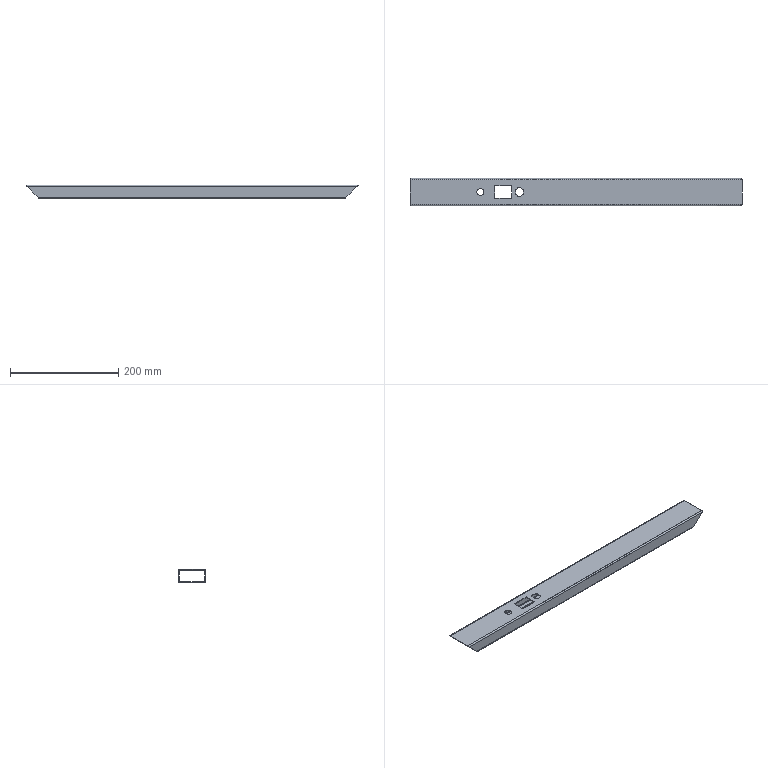Part | STEP file | 6150502 | 1 solid | 31 faces | box 613 x 50 x 25 mm | volume 116984 mm3 | plane 20 | cylinder 11 | commonest cylinder face diameters 2 x4 5 x4 15.8 x2 13 x1
STEP:
#1=CARTESIAN_POINT('',(-284.,-25.,-10.));
#2=VERTEX_POINT('',#1);
#3=CARTESIAN_POINT('',(284.,-25.,-10.));
#4=VERTEX_POINT('',#3);
#5=CARTESIAN_POINT('',(-306.5,-25.,-10.));
#6=DIRECTION('',(1.,0.,0.));
#7=VECTOR('',#6,1000.);
#8=LINE('',#5,#7);
#9=EDGE_CURVE('',#2,#4,#8,.T.);
#10=ORIENTED_EDGE('',*,*,#9,.T.);
#11=CARTESIAN_POINT('',(304.,-25.,10.));
#12=VERTEX_POINT('',#11);
#13=CARTESIAN_POINT('',(306.5,-25.,12.5));
#14=DIRECTION('',(0.7071,0.,0.7071));
#15=VECTOR('',#14,1000.);
#16=LINE('',#13,#15);
#17=EDGE_CURVE('',#4,#12,#16,.T.);
#18=ORIENTED_EDGE('',*,*,#17,.T.);
#19=CARTESIAN_POINT('',(-304.,-25.,10.));
#20=VERTEX_POINT('',#19);
#21=CARTESIAN_POINT('',(-306.5,-25.,10.));
#22=DIRECTION('',(-1.,0.,0.));
#23=VECTOR('',#22,1000.);
#24=LINE('',#21,#23);
#25=EDGE_CURVE('',#12,#20,#24,.T.);
#26=ORIENTED_EDGE('',*,*,#25,.T.);
#27=CARTESIAN_POINT('',(-306.5,-25.,12.5));
#28=DIRECTION('',(0.7071,0.,-0.7071));
#29=VECTOR('',#28,1000.);
#30=LINE('',#27,#29);
#31=EDGE_CURVE('',#20,#2,#30,.T.);
#32=ORIENTED_EDGE('',*,*,#31,.T.);
#33=EDGE_LOOP('',(#10,#18,#26,#32));
#34=FACE_OUTER_BOUND('',#33,.T.);
#35=CARTESIAN_POINT('',(-306.5,-25.,12.5));
#36=DIRECTION('',(0.,1.,0.));
#37=DIRECTION('',(-1.,0.,0.));
#38=AXIS2_PLACEMENT_3D('',#35,#36,#37);
#39=PLANE('',#38);
#40=ADVANCED_FACE('',(#34),#39,.F.);
#41=CARTESIAN_POINT('',(-304.,25.,10.));
#42=VERTEX_POINT('',#41);
#43=CARTESIAN_POINT('',(304.,25.,10.));
#44=VERTEX_POINT('',#43);
#45=CARTESIAN_POINT('',(306.5,25.,10.));
#46=DIRECTION('',(1.,0.,0.));
#47=VECTOR('',#46,1000.);
#48=LINE('',#45,#47);
#49=EDGE_CURVE('',#42,#44,#48,.T.);
#50=ORIENTED_EDGE('',*,*,#49,.T.);
#51=CARTESIAN_POINT('',(284.,25.,-10.));
#52=VERTEX_POINT('',#51);
#53=CARTESIAN_POINT('',(306.5,25.,12.5));
#54=DIRECTION('',(0.7071,0.,0.7071));
#55=VECTOR('',#54,1000.);
#56=LINE('',#53,#55);
#57=EDGE_CURVE('',#52,#44,#56,.T.);
#58=ORIENTED_EDGE('',*,*,#57,.F.);
#59=CARTESIAN_POINT('',(-284.,25.,-10.));
#60=VERTEX_POINT('',#59);
#61=CARTESIAN_POINT('',(-306.5,25.,-10.));
#62=DIRECTION('',(-1.,0.,0.));
#63=VECTOR('',#62,1000.);
#64=LINE('',#61,#63);
#65=EDGE_CURVE('',#52,#60,#64,.T.);
#66=ORIENTED_EDGE('',*,*,#65,.T.);
#67=CARTESIAN_POINT('',(-306.5,25.,12.5));
#68=DIRECTION('',(0.7071,0.,-0.7071));
#69=VECTOR('',#68,1000.);
#70=LINE('',#67,#69);
#71=EDGE_CURVE('',#42,#60,#70,.T.);
#72=ORIENTED_EDGE('',*,*,#71,.F.);
#73=EDGE_LOOP('',(#50,#58,#66,#72));
#74=FACE_OUTER_BOUND('',#73,.T.);
#75=CARTESIAN_POINT('',(-306.5,25.,12.5));
#76=DIRECTION('',(0.,-1.,0.));
#77=DIRECTION('',(0.,0.,-1.));
#78=AXIS2_PLACEMENT_3D('',#75,#76,#77);
#79=PLANE('',#78);
#80=ADVANCED_FACE('',(#74),#79,.F.);
#81=CARTESIAN_POINT('',(-111.4,-3.847,12.5));
#82=VERTEX_POINT('',#81);
#83=CARTESIAN_POINT('',(-97.6,-3.847,12.5));
#84=VERTEX_POINT('',#83);
#85=CARTESIAN_POINT('',(-104.5,0.,12.5));
#86=DIRECTION('',(0.,0.,1.));
#87=DIRECTION('',(1.,0.,0.));
#88=AXIS2_PLACEMENT_3D('',#85,#86,#87);
#89=CIRCLE('',#88,7.9);
#90=EDGE_CURVE('',#82,#84,#89,.T.);
#91=ORIENTED_EDGE('',*,*,#90,.F.);
#92=CARTESIAN_POINT('',(-111.4,3.847,12.5));
#93=VERTEX_POINT('',#92);
#94=CARTESIAN_POINT('',(-111.4,-3.847,12.5));
#95=DIRECTION('',(0.,-1.,0.));
#96=VECTOR('',#95,1000.);
#97=LINE('',#94,#96);
#98=EDGE_CURVE('',#93,#82,#97,.T.);
#99=ORIENTED_EDGE('',*,*,#98,.F.);
#100=CARTESIAN_POINT('',(-97.6,3.847,12.5));
#101=VERTEX_POINT('',#100);
#102=CARTESIAN_POINT('',(-104.5,0.,12.5));
#103=DIRECTION('',(0.,0.,1.));
#104=DIRECTION('',(1.,0.,0.));
#105=AXIS2_PLACEMENT_3D('',#102,#103,#104);
#106=CIRCLE('',#105,7.9);
#107=EDGE_CURVE('',#101,#93,#106,.T.);
#108=ORIENTED_EDGE('',*,*,#107,.F.);
#109=CARTESIAN_POINT('',(-97.6,3.847,12.5));
#110=DIRECTION('',(0.,1.,0.));
#111=VECTOR('',#110,1000.);
#112=LINE('',#109,#111);
#113=EDGE_CURVE('',#84,#101,#112,.T.);
#114=ORIENTED_EDGE('',*,*,#113,.F.);
#115=EDGE_LOOP('',(#91,#99,#108,#114));
#116=FACE_BOUND('',#115,.T.);
#117=CARTESIAN_POINT('',(-150.,11.25,12.5));
#118=VERTEX_POINT('',#117);
#119=CARTESIAN_POINT('',(-150.,-11.25,12.5));
#120=VERTEX_POINT('',#119);
#121=CARTESIAN_POINT('',(-150.,11.25,12.5));
#122=DIRECTION('',(0.,-1.,0.));
#123=VECTOR('',#122,1000.);
#124=LINE('',#121,#123);
#125=EDGE_CURVE('',#118,#120,#124,.T.);
#126=ORIENTED_EDGE('',*,*,#125,.F.);
#127=CARTESIAN_POINT('',(-119.,11.25,12.5));
#128=VERTEX_POINT('',#127);
#129=CARTESIAN_POINT('',(-150.,11.25,12.5));
#130=DIRECTION('',(-1.,0.,0.));
#131=VECTOR('',#130,1000.);
#132=LINE('',#129,#131);
#133=EDGE_CURVE('',#128,#118,#132,.T.);
#134=ORIENTED_EDGE('',*,*,#133,.F.);
#135=CARTESIAN_POINT('',(-119.,-11.25,12.5));
#136=VERTEX_POINT('',#135);
#137=CARTESIAN_POINT('',(-119.,11.25,12.5));
#138=DIRECTION('',(0.,1.,0.));
#139=VECTOR('',#138,1000.);
#140=LINE('',#137,#139);
#141=EDGE_CURVE('',#136,#128,#140,.T.);
#142=ORIENTED_EDGE('',*,*,#141,.F.);
#143=CARTESIAN_POINT('',(-150.,-11.25,12.5));
#144=DIRECTION('',(1.,0.,0.));
#145=VECTOR('',#144,1000.);
#146=LINE('',#143,#145);
#147=EDGE_CURVE('',#120,#136,#146,.T.);
#148=ORIENTED_EDGE('',*,*,#147,.F.);
#149=EDGE_LOOP('',(#126,#134,#142,#148));
#150=FACE_BOUND('',#149,.T.);
#151=CARTESIAN_POINT('',(-170.,0.,12.5));
#152=VERTEX_POINT('',#151);
#153=CARTESIAN_POINT('',(-176.5,0.,12.5));
#154=DIRECTION('',(0.,0.,1.));
#155=DIRECTION('',(1.,0.,0.));
#156=AXIS2_PLACEMENT_3D('',#153,#154,#155);
#157=CIRCLE('',#156,6.5);
#158=EDGE_CURVE('',#152,#152,#157,.T.);
#159=ORIENTED_EDGE('',*,*,#158,.F.);
#160=EDGE_LOOP('',(#159));
#161=FACE_BOUND('',#160,.T.);
#162=CARTESIAN_POINT('',(-306.5,22.5,12.5));
#163=VERTEX_POINT('',#162);
#164=CARTESIAN_POINT('',(-306.5,-22.5,12.5));
#165=VERTEX_POINT('',#164);
#166=CARTESIAN_POINT('',(-306.5,25.,12.5));
#167=DIRECTION('',(0.,-1.,0.));
#168=VECTOR('',#167,1000.);
#169=LINE('',#166,#168);
#170=EDGE_CURVE('',#163,#165,#169,.T.);
#171=ORIENTED_EDGE('',*,*,#170,.T.);
#172=CARTESIAN_POINT('',(306.5,-22.5,12.5));
#173=VERTEX_POINT('',#172);
#174=CARTESIAN_POINT('',(306.5,-22.5,12.5));
#175=DIRECTION('',(1.,0.,0.));
#176=VECTOR('',#175,1000.);
#177=LINE('',#174,#176);
#178=EDGE_CURVE('',#165,#173,#177,.T.);
#179=ORIENTED_EDGE('',*,*,#178,.T.);
#180=CARTESIAN_POINT('',(306.5,22.5,12.5));
#181=VERTEX_POINT('',#180);
#182=CARTESIAN_POINT('',(306.5,25.,12.5));
#183=DIRECTION('',(0.,1.,0.));
#184=VECTOR('',#183,1000.);
#185=LINE('',#182,#184);
#186=EDGE_CURVE('',#173,#181,#185,.T.);
#187=ORIENTED_EDGE('',*,*,#186,.T.);
#188=CARTESIAN_POINT('',(-306.5,22.5,12.5));
#189=DIRECTION('',(-1.,0.,0.));
#190=VECTOR('',#189,1000.);
#191=LINE('',#188,#190);
#192=EDGE_CURVE('',#181,#163,#191,.T.);
#193=ORIENTED_EDGE('',*,*,#192,.T.);
#194=EDGE_LOOP('',(#171,#179,#187,#193));
#195=FACE_OUTER_BOUND('',#194,.T.);
#196=CARTESIAN_POINT('',(-306.5,25.,12.5));
#197=DIRECTION('',(0.,0.,1.));
#198=DIRECTION('',(1.,0.,0.));
#199=AXIS2_PLACEMENT_3D('',#196,#197,#198);
#200=PLANE('',#199);
#201=ADVANCED_FACE('',(#116,#150,#161,#195),#200,.T.);
#202=CARTESIAN_POINT('',(-76.5,-15.,-12.5));
#203=VERTEX_POINT('',#202);
#204=CARTESIAN_POINT('',(-206.5,-15.,-12.5));
#205=VERTEX_POINT('',#204);
#206=CARTESIAN_POINT('',(-76.5,-15.,-12.5));
#207=DIRECTION('',(-1.,0.,0.));
#208=VECTOR('',#207,1000.);
#209=LINE('',#206,#208);
#210=EDGE_CURVE('',#203,#205,#209,.T.);
#211=ORIENTED_EDGE('',*,*,#210,.F.);
#212=CARTESIAN_POINT('',(-76.5,15.,-12.5));
#213=VERTEX_POINT('',#212);
#214=CARTESIAN_POINT('',(-76.5,15.,-12.5));
#215=DIRECTION('',(0.,-1.,0.));
#216=VECTOR('',#215,1000.);
#217=LINE('',#214,#216);
#218=EDGE_CURVE('',#213,#203,#217,.T.);
#219=ORIENTED_EDGE('',*,*,#218,.F.);
#220=CARTESIAN_POINT('',(-206.5,15.,-12.5));
#221=VERTEX_POINT('',#220);
#222=CARTESIAN_POINT('',(-76.5,15.,-12.5));
#223=DIRECTION('',(1.,0.,0.));
#224=VECTOR('',#223,1000.);
#225=LINE('',#222,#224);
#226=EDGE_CURVE('',#221,#213,#225,.T.);
#227=ORIENTED_EDGE('',*,*,#226,.F.);
#228=CARTESIAN_POINT('',(-206.5,15.,-12.5));
#229=DIRECTION('',(0.,1.,0.));
#230=VECTOR('',#229,1000.);
#231=LINE('',#228,#230);
#232=EDGE_CURVE('',#205,#221,#231,.T.);
#233=ORIENTED_EDGE('',*,*,#232,.F.);
#234=EDGE_LOOP('',(#211,#219,#227,#233));
#235=FACE_BOUND('',#234,.T.);
#236=CARTESIAN_POINT('',(-281.5,22.5,-12.5));
#237=VERTEX_POINT('',#236);
#238=CARTESIAN_POINT('',(281.5,22.5,-12.5));
#239=VERTEX_POINT('',#238);
#240=CARTESIAN_POINT('',(-306.5,22.5,-12.5));
#241=DIRECTION('',(1.,0.,0.));
#242=VECTOR('',#241,1000.);
#243=LINE('',#240,#242);
#244=EDGE_CURVE('',#237,#239,#243,.T.);
#245=ORIENTED_EDGE('',*,*,#244,.T.);
#246=CARTESIAN_POINT('',(281.5,-22.5,-12.5));
#247=VERTEX_POINT('',#246);
#248=CARTESIAN_POINT('',(281.5,25.,-12.5));
#249=DIRECTION('',(0.,-1.,0.));
#250=VECTOR('',#249,1000.);
#251=LINE('',#248,#250);
#252=EDGE_CURVE('',#239,#247,#251,.T.);
#253=ORIENTED_EDGE('',*,*,#252,.T.);
#254=CARTESIAN_POINT('',(-281.5,-22.5,-12.5));
#255=VERTEX_POINT('',#254);
#256=CARTESIAN_POINT('',(-306.5,-22.5,-12.5));
#257=DIRECTION('',(-1.,0.,0.));
#258=VECTOR('',#257,1000.);
#259=LINE('',#256,#258);
#260=EDGE_CURVE('',#247,#255,#259,.T.);
#261=ORIENTED_EDGE('',*,*,#260,.T.);
#262=CARTESIAN_POINT('',(-281.5,25.,-12.5));
#263=DIRECTION('',(0.,1.,0.));
#264=VECTOR('',#263,1000.);
#265=LINE('',#262,#264);
#266=EDGE_CURVE('',#255,#237,#265,.T.);
#267=ORIENTED_EDGE('',*,*,#266,.T.);
#268=EDGE_LOOP('',(#245,#253,#261,#267));
#269=FACE_OUTER_BOUND('',#268,.T.);
#270=CARTESIAN_POINT('',(-306.5,25.,-12.5));
#271=DIRECTION('',(0.,0.,1.));
#272=DIRECTION('',(1.,0.,0.));
#273=AXIS2_PLACEMENT_3D('',#270,#271,#272);
#274=PLANE('',#273);
#275=ADVANCED_FACE('',(#235,#269),#274,.F.);
#276=CARTESIAN_POINT('',(306.5,-22.5,12.5));
#277=CARTESIAN_POINT('',(306.5,-23.964,12.5));
#278=CARTESIAN_POINT('',(305.464,-25.,11.464));
#279=CARTESIAN_POINT('',(304.,-25.,10.));
#280=(BOUNDED_CURVE()B_SPLINE_CURVE(3,(#276,#277,#278,#279),.UNSPECIFIED.,.F.,.F.)B_SPLINE_CURVE_WITH_KNOTS((4,4),(3.142,4.712),.UNSPECIFIED.)CURVE()GEOMETRIC_REPRESENTATION_ITEM()RATIONAL_B_SPLINE_CURVE((1.,0.8047,0.8047,1.))REPRESENTATION_ITEM(''));
#281=EDGE_CURVE('',#173,#12,#280,.T.);
#282=ORIENTED_EDGE('',*,*,#281,.F.);
#283=ORIENTED_EDGE('',*,*,#178,.F.);
#284=CARTESIAN_POINT('',(-304.,-25.,10.));
#285=CARTESIAN_POINT('',(-305.464,-25.,11.464));
#286=CARTESIAN_POINT('',(-306.5,-23.964,12.5));
#287=CARTESIAN_POINT('',(-306.5,-22.5,12.5));
#288=(BOUNDED_CURVE()B_SPLINE_CURVE(3,(#284,#285,#286,#287),.UNSPECIFIED.,.F.,.F.)B_SPLINE_CURVE_WITH_KNOTS((4,4),(4.712,6.283),.UNSPECIFIED.)CURVE()GEOMETRIC_REPRESENTATION_ITEM()RATIONAL_B_SPLINE_CURVE((1.,0.8047,0.8047,1.))REPRESENTATION_ITEM(''));
#289=EDGE_CURVE('',#20,#165,#288,.T.);
#290=ORIENTED_EDGE('',*,*,#289,.F.);
#291=ORIENTED_EDGE('',*,*,#25,.F.);
#292=EDGE_LOOP('',(#282,#283,#290,#291));
#293=FACE_OUTER_BOUND('',#292,.T.);
#294=CARTESIAN_POINT('',(-306.5,-22.5,10.));
#295=DIRECTION('',(-1.,0.,0.));
#296=DIRECTION('',(0.,-1.,0.));
#297=AXIS2_PLACEMENT_3D('',#294,#295,#296);
#298=CYLINDRICAL_SURFACE('',#297,2.5);
#299=ADVANCED_FACE('',(#293),#298,.T.);
#300=CARTESIAN_POINT('',(284.,-25.,-10.));
#301=CARTESIAN_POINT('',(282.536,-25.,-11.464));
#302=CARTESIAN_POINT('',(281.5,-23.964,-12.5));
#303=CARTESIAN_POINT('',(281.5,-22.5,-12.5));
#304=(BOUNDED_CURVE()B_SPLINE_CURVE(3,(#300,#301,#302,#303),.UNSPECIFIED.,.F.,.F.)B_SPLINE_CURVE_WITH_KNOTS((4,4),(1.571,3.142),.UNSPECIFIED.)CURVE()GEOMETRIC_REPRESENTATION_ITEM()RATIONAL_B_SPLINE_CURVE((1.,0.8047,0.8047,1.))REPRESENTATION_ITEM(''));
#305=EDGE_CURVE('',#4,#247,#304,.T.);
#306=ORIENTED_EDGE('',*,*,#305,.F.);
#307=ORIENTED_EDGE('',*,*,#9,.F.);
#308=CARTESIAN_POINT('',(-281.5,-22.5,-12.5));
#309=CARTESIAN_POINT('',(-281.5,-23.964,-12.5));
#310=CARTESIAN_POINT('',(-282.536,-25.,-11.464));
#311=CARTESIAN_POINT('',(-284.,-25.,-10.));
#312=(BOUNDED_CURVE()B_SPLINE_CURVE(3,(#308,#309,#310,#311),.UNSPECIFIED.,.F.,.F.)B_SPLINE_CURVE_WITH_KNOTS((4,4),(0.,1.571),.UNSPECIFIED.)CURVE()GEOMETRIC_REPRESENTATION_ITEM()RATIONAL_B_SPLINE_CURVE((1.,0.8047,0.8047,1.))REPRESENTATION_ITEM(''));
#313=EDGE_CURVE('',#255,#2,#312,.T.);
#314=ORIENTED_EDGE('',*,*,#313,.F.);
#315=ORIENTED_EDGE('',*,*,#260,.F.);
#316=EDGE_LOOP('',(#306,#307,#314,#315));
#317=FACE_OUTER_BOUND('',#316,.T.);
#318=CARTESIAN_POINT('',(-306.5,-22.5,-10.));
#319=DIRECTION('',(1.,0.,0.));
#320=DIRECTION('',(0.,1.,0.));
#321=AXIS2_PLACEMENT_3D('',#318,#319,#320);
#322=CYLINDRICAL_SURFACE('',#321,2.5);
#323=ADVANCED_FACE('',(#317),#322,.T.);
#324=CARTESIAN_POINT('',(281.5,22.5,-12.5));
#325=CARTESIAN_POINT('',(281.5,23.964,-12.5));
#326=CARTESIAN_POINT('',(282.536,25.,-11.464));
#327=CARTESIAN_POINT('',(284.,25.,-10.));
#328=(BOUNDED_CURVE()B_SPLINE_CURVE(3,(#324,#325,#326,#327),.UNSPECIFIED.,.F.,.F.)B_SPLINE_CURVE_WITH_KNOTS((4,4),(0.,1.571),.UNSPECIFIED.)CURVE()GEOMETRIC_REPRESENTATION_ITEM()RATIONAL_B_SPLINE_CURVE((1.,0.8047,0.8047,1.))REPRESENTATION_ITEM(''));
#329=EDGE_CURVE('',#239,#52,#328,.T.);
#330=ORIENTED_EDGE('',*,*,#329,.F.);
#331=ORIENTED_EDGE('',*,*,#244,.F.);
#332=CARTESIAN_POINT('',(-284.,25.,-10.));
#333=CARTESIAN_POINT('',(-282.536,25.,-11.464));
#334=CARTESIAN_POINT('',(-281.5,23.964,-12.5));
#335=CARTESIAN_POINT('',(-281.5,22.5,-12.5));
#336=(BOUNDED_CURVE()B_SPLINE_CURVE(3,(#332,#333,#334,#335),.UNSPECIFIED.,.F.,.T.)B_SPLINE_CURVE_WITH_KNOTS((4,4),(1.571,3.142),.UNSPECIFIED.)CURVE()GEOMETRIC_REPRESENTATION_ITEM()RATIONAL_B_SPLINE_CURVE((1.,0.8047,0.8047,1.))REPRESENTATION_ITEM(''));
#337=EDGE_CURVE('',#60,#237,#336,.T.);
#338=ORIENTED_EDGE('',*,*,#337,.F.);
#339=ORIENTED_EDGE('',*,*,#65,.F.);
#340=EDGE_LOOP('',(#330,#331,#338,#339));
#341=FACE_OUTER_BOUND('',#340,.T.);
#342=CARTESIAN_POINT('',(-306.5,22.5,-10.));
#343=DIRECTION('',(-1.,0.,0.));
#344=DIRECTION('',(0.,0.,1.));
#345=AXIS2_PLACEMENT_3D('',#342,#343,#344);
#346=CYLINDRICAL_SURFACE('',#345,2.5);
#347=ADVANCED_FACE('',(#341),#346,.T.);
#348=CARTESIAN_POINT('',(304.,25.,10.));
#349=CARTESIAN_POINT('',(305.464,25.,11.464));
#350=CARTESIAN_POINT('',(306.5,23.964,12.5));
#351=CARTESIAN_POINT('',(306.5,22.5,12.5));
#352=(BOUNDED_CURVE()B_SPLINE_CURVE(3,(#348,#349,#350,#351),.UNSPECIFIED.,.F.,.F.)B_SPLINE_CURVE_WITH_KNOTS((4,4),(4.712,6.283),.UNSPECIFIED.)CURVE()GEOMETRIC_REPRESENTATION_ITEM()RATIONAL_B_SPLINE_CURVE((1.,0.8047,0.8047,1.))REPRESENTATION_ITEM(''));
#353=EDGE_CURVE('',#44,#181,#352,.T.);
#354=ORIENTED_EDGE('',*,*,#353,.F.);
#355=ORIENTED_EDGE('',*,*,#49,.F.);
#356=CARTESIAN_POINT('',(-306.5,22.5,12.5));
#357=CARTESIAN_POINT('',(-306.5,23.964,12.5));
#358=CARTESIAN_POINT('',(-305.464,25.,11.464));
#359=CARTESIAN_POINT('',(-304.,25.,10.));
#360=(BOUNDED_CURVE()B_SPLINE_CURVE(3,(#356,#357,#358,#359),.UNSPECIFIED.,.F.,.F.)B_SPLINE_CURVE_WITH_KNOTS((4,4),(3.142,4.712),.UNSPECIFIED.)CURVE()GEOMETRIC_REPRESENTATION_ITEM()RATIONAL_B_SPLINE_CURVE((1.,0.8047,0.8047,1.))REPRESENTATION_ITEM(''));
#361=EDGE_CURVE('',#163,#42,#360,.T.);
#362=ORIENTED_EDGE('',*,*,#361,.F.);
#363=ORIENTED_EDGE('',*,*,#192,.F.);
#364=EDGE_LOOP('',(#354,#355,#362,#363));
#365=FACE_OUTER_BOUND('',#364,.T.);
#366=CARTESIAN_POINT('',(-306.5,22.5,10.));
#367=DIRECTION('',(1.,0.,0.));
#368=DIRECTION('',(0.,0.,-1.));
#369=AXIS2_PLACEMENT_3D('',#366,#367,#368);
#370=CYLINDRICAL_SURFACE('',#369,2.5);
#371=ADVANCED_FACE('',(#365),#370,.T.);
#372=CARTESIAN_POINT('',(284.,-23.5,-10.));
#373=VERTEX_POINT('',#372);
#374=CARTESIAN_POINT('',(304.,-23.5,10.));
#375=VERTEX_POINT('',#374);
#376=CARTESIAN_POINT('',(0.,-23.5,-294.));
#377=DIRECTION('',(0.7071,0.,0.7071));
#378=VECTOR('',#377,1000.);
#379=LINE('',#376,#378);
#380=EDGE_CURVE('',#373,#375,#379,.T.);
#381=ORIENTED_EDGE('',*,*,#380,.F.);
#382=CARTESIAN_POINT('',(-284.,-23.5,-10.));
#383=VERTEX_POINT('',#382);
#384=CARTESIAN_POINT('',(-306.5,-23.5,-10.));
#385=DIRECTION('',(1.,0.,0.));
#386=VECTOR('',#385,1000.);
#387=LINE('',#384,#386);
#388=EDGE_CURVE('',#383,#373,#387,.T.);
#389=ORIENTED_EDGE('',*,*,#388,.F.);
#390=CARTESIAN_POINT('',(-304.,-23.5,10.));
#391=VERTEX_POINT('',#390);
#392=CARTESIAN_POINT('',(-306.5,-23.5,12.5));
#393=DIRECTION('',(0.7071,0.,-0.7071));
#394=VECTOR('',#393,1000.);
#395=LINE('',#392,#394);
#396=EDGE_CURVE('',#391,#383,#395,.T.);
#397=ORIENTED_EDGE('',*,*,#396,.F.);
#398=CARTESIAN_POINT('',(-306.5,-23.5,10.));
#399=DIRECTION('',(-1.,0.,0.));
#400=VECTOR('',#399,1000.);
#401=LINE('',#398,#400);
#402=EDGE_CURVE('',#375,#391,#401,.T.);
#403=ORIENTED_EDGE('',*,*,#402,.F.);
#404=EDGE_LOOP('',(#381,#389,#397,#403));
#405=FACE_OUTER_BOUND('',#404,.T.);
#406=CARTESIAN_POINT('',(-306.5,-23.5,12.5));
#407=DIRECTION('',(0.,1.,0.));
#408=DIRECTION('',(-1.,0.,0.));
#409=AXIS2_PLACEMENT_3D('',#406,#407,#408);
#410=PLANE('',#409);
#411=ADVANCED_FACE('',(#405),#410,.T.);
#412=CARTESIAN_POINT('',(304.,23.5,10.));
#413=VERTEX_POINT('',#412);
#414=CARTESIAN_POINT('',(284.,23.5,-10.));
#415=VERTEX_POINT('',#414);
#416=CARTESIAN_POINT('',(0.,23.5,-294.));
#417=DIRECTION('',(-0.7071,0.,-0.7071));
#418=VECTOR('',#417,1000.);
#419=LINE('',#416,#418);
#420=EDGE_CURVE('',#413,#415,#419,.T.);
#421=ORIENTED_EDGE('',*,*,#420,.F.);
#422=CARTESIAN_POINT('',(-304.,23.5,10.));
#423=VERTEX_POINT('',#422);
#424=CARTESIAN_POINT('',(-306.5,23.5,10.));
#425=DIRECTION('',(1.,0.,0.));
#426=VECTOR('',#425,1000.);
#427=LINE('',#424,#426);
#428=EDGE_CURVE('',#423,#413,#427,.T.);
#429=ORIENTED_EDGE('',*,*,#428,.F.);
#430=CARTESIAN_POINT('',(-284.,23.5,-10.));
#431=VERTEX_POINT('',#430);
#432=CARTESIAN_POINT('',(-306.5,23.5,12.5));
#433=DIRECTION('',(-0.7071,0.,0.7071));
#434=VECTOR('',#433,1000.);
#435=LINE('',#432,#434);
#436=EDGE_CURVE('',#431,#423,#435,.T.);
#437=ORIENTED_EDGE('',*,*,#436,.F.);
#438=CARTESIAN_POINT('',(-306.5,23.5,-10.));
#439=DIRECTION('',(-1.,0.,0.));
#440=VECTOR('',#439,1000.);
#441=LINE('',#438,#440);
#442=EDGE_CURVE('',#415,#431,#441,.T.);
#443=ORIENTED_EDGE('',*,*,#442,.F.);
#444=EDGE_LOOP('',(#421,#429,#437,#443));
#445=FACE_OUTER_BOUND('',#444,.T.);
#446=CARTESIAN_POINT('',(-306.5,23.5,12.5));
#447=DIRECTION('',(0.,-1.,0.));
#448=DIRECTION('',(0.,0.,-1.));
#449=AXIS2_PLACEMENT_3D('',#446,#447,#448);
#450=PLANE('',#449);
#451=ADVANCED_FACE('',(#445),#450,.T.);
#452=CARTESIAN_POINT('',(-111.4,3.847,11.));
#453=VERTEX_POINT('',#452);
#454=CARTESIAN_POINT('',(-111.4,-3.847,11.));
#455=VERTEX_POINT('',#454);
#456=CARTESIAN_POINT('',(-111.4,25.,11.));
#457=DIRECTION('',(0.,-1.,0.));
#458=VECTOR('',#457,1000.);
#459=LINE('',#456,#458);
#460=EDGE_CURVE('',#453,#455,#459,.T.);
#461=ORIENTED_EDGE('',*,*,#460,.T.);
#462=CARTESIAN_POINT('',(-97.6,-3.847,11.));
#463=VERTEX_POINT('',#462);
#464=CARTESIAN_POINT('',(-104.5,0.,11.));
#465=DIRECTION('',(0.,0.,1.));
#466=DIRECTION('',(1.,0.,0.));
#467=AXIS2_PLACEMENT_3D('',#464,#465,#466);
#468=CIRCLE('',#467,7.9);
#469=EDGE_CURVE('',#455,#463,#468,.T.);
#470=ORIENTED_EDGE('',*,*,#469,.T.);
#471=CARTESIAN_POINT('',(-97.6,3.847,11.));
#472=VERTEX_POINT('',#471);
#473=CARTESIAN_POINT('',(-97.6,25.,11.));
#474=DIRECTION('',(0.,1.,0.));
#475=VECTOR('',#474,1000.);
#476=LINE('',#473,#475);
#477=EDGE_CURVE('',#463,#472,#476,.T.);
#478=ORIENTED_EDGE('',*,*,#477,.T.);
#479=CARTESIAN_POINT('',(-104.5,0.,11.));
#480=DIRECTION('',(0.,0.,1.));
#481=DIRECTION('',(1.,0.,0.));
#482=AXIS2_PLACEMENT_3D('',#479,#480,#481);
#483=CIRCLE('',#482,7.9);
#484=EDGE_CURVE('',#472,#453,#483,.T.);
#485=ORIENTED_EDGE('',*,*,#484,.T.);
#486=EDGE_LOOP('',(#461,#470,#478,#485));
#487=FACE_BOUND('',#486,.T.);
#488=CARTESIAN_POINT('',(-119.,11.25,11.));
#489=VERTEX_POINT('',#488);
#490=CARTESIAN_POINT('',(-150.,11.25,11.));
#491=VERTEX_POINT('',#490);
#492=CARTESIAN_POINT('',(-306.5,11.25,11.));
#493=DIRECTION('',(-1.,0.,0.));
#494=VECTOR('',#493,1000.);
#495=LINE('',#492,#494);
#496=EDGE_CURVE('',#489,#491,#495,.T.);
#497=ORIENTED_EDGE('',*,*,#496,.T.);
#498=CARTESIAN_POINT('',(-150.,-11.25,11.));
#499=VERTEX_POINT('',#498);
#500=CARTESIAN_POINT('',(-150.,25.,11.));
#501=DIRECTION('',(0.,-1.,0.));
#502=VECTOR('',#501,1000.);
#503=LINE('',#500,#502);
#504=EDGE_CURVE('',#491,#499,#503,.T.);
#505=ORIENTED_EDGE('',*,*,#504,.T.);
#506=CARTESIAN_POINT('',(-119.,-11.25,11.));
#507=VERTEX_POINT('',#506);
#508=CARTESIAN_POINT('',(-306.5,-11.25,11.));
#509=DIRECTION('',(1.,0.,0.));
#510=VECTOR('',#509,1000.);
#511=LINE('',#508,#510);
#512=EDGE_CURVE('',#499,#507,#511,.T.);
#513=ORIENTED_EDGE('',*,*,#512,.T.);
#514=CARTESIAN_POINT('',(-119.,25.,11.));
#515=DIRECTION('',(0.,1.,0.));
#516=VECTOR('',#515,1000.);
#517=LINE('',#514,#516);
#518=EDGE_CURVE('',#507,#489,#517,.T.);
#519=ORIENTED_EDGE('',*,*,#518,.T.);
#520=EDGE_LOOP('',(#497,#505,#513,#519));
#521=FACE_BOUND('',#520,.T.);
#522=CARTESIAN_POINT('',(-170.,0.,11.));
#523=VERTEX_POINT('',#522);
#524=CARTESIAN_POINT('',(-176.5,0.,11.));
#525=DIRECTION('',(0.,0.,1.));
#526=DIRECTION('',(1.,0.,0.));
#527=AXIS2_PLACEMENT_3D('',#524,#525,#526);
#528=CIRCLE('',#527,6.5);
#529=EDGE_CURVE('',#523,#523,#528,.T.);
#530=ORIENTED_EDGE('',*,*,#529,.T.);
#531=EDGE_LOOP('',(#530));
#532=FACE_BOUND('',#531,.T.);
#533=CARTESIAN_POINT('',(305.,22.5,11.));
#534=VERTEX_POINT('',#533);
#535=CARTESIAN_POINT('',(-305.,22.5,11.));
#536=VERTEX_POINT('',#535);
#537=CARTESIAN_POINT('',(-306.5,22.5,11.));
#538=DIRECTION('',(-1.,0.,0.));
#539=VECTOR('',#538,1000.);
#540=LINE('',#537,#539);
#541=EDGE_CURVE('',#534,#536,#540,.T.);
#542=ORIENTED_EDGE('',*,*,#541,.F.);
#543=CARTESIAN_POINT('',(305.,-22.5,11.));
#544=VERTEX_POINT('',#543);
#545=CARTESIAN_POINT('',(305.,25.,11.));
#546=DIRECTION('',(0.,-1.,0.));
#547=VECTOR('',#546,1000.);
#548=LINE('',#545,#547);
#549=EDGE_CURVE('',#534,#544,#548,.T.);
#550=ORIENTED_EDGE('',*,*,#549,.T.);
#551=CARTESIAN_POINT('',(-305.,-22.5,11.));
#552=VERTEX_POINT('',#551);
#553=CARTESIAN_POINT('',(-306.5,-22.5,11.));
#554=DIRECTION('',(1.,0.,0.));
#555=VECTOR('',#554,1000.);
#556=LINE('',#553,#555);
#557=EDGE_CURVE('',#552,#544,#556,.T.);
#558=ORIENTED_EDGE('',*,*,#557,.F.);
#559=CARTESIAN_POINT('',(-305.,25.,11.));
#560=DIRECTION('',(0.,1.,0.));
#561=VECTOR('',#560,1000.);
#562=LINE('',#559,#561);
#563=EDGE_CURVE('',#552,#536,#562,.T.);
#564=ORIENTED_EDGE('',*,*,#563,.T.);
#565=EDGE_LOOP('',(#542,#550,#558,#564));
#566=FACE_OUTER_BOUND('',#565,.T.);
#567=CARTESIAN_POINT('',(-306.5,25.,11.));
#568=DIRECTION('',(0.,0.,1.));
#569=DIRECTION('',(1.,0.,0.));
#570=AXIS2_PLACEMENT_3D('',#567,#568,#569);
#571=PLANE('',#570);
#572=ADVANCED_FACE('',(#487,#521,#532,#566),#571,.F.);
#573=CARTESIAN_POINT('',(-76.5,-15.,-11.));
#574=VERTEX_POINT('',#573);
#575=CARTESIAN_POINT('',(-76.5,15.,-11.));
#576=VERTEX_POINT('',#575);
#577=CARTESIAN_POINT('',(-76.5,25.,-11.));
#578=DIRECTION('',(0.,1.,0.));
#579=VECTOR('',#578,1000.);
#580=LINE('',#577,#579);
#581=EDGE_CURVE('',#574,#576,#580,.T.);
#582=ORIENTED_EDGE('',*,*,#581,.F.);
#583=CARTESIAN_POINT('',(-206.5,-15.,-11.));
#584=VERTEX_POINT('',#583);
#585=CARTESIAN_POINT('',(-306.5,-15.,-11.));
#586=DIRECTION('',(1.,0.,0.));
#587=VECTOR('',#586,1000.);
#588=LINE('',#585,#587);
#589=EDGE_CURVE('',#584,#574,#588,.T.);
#590=ORIENTED_EDGE('',*,*,#589,.F.);
#591=CARTESIAN_POINT('',(-206.5,15.,-11.));
#592=VERTEX_POINT('',#591);
#593=CARTESIAN_POINT('',(-206.5,25.,-11.));
#594=DIRECTION('',(0.,-1.,0.));
#595=VECTOR('',#594,1000.);
#596=LINE('',#593,#595);
#597=EDGE_CURVE('',#592,#584,#596,.T.);
#598=ORIENTED_EDGE('',*,*,#597,.F.);
#599=CARTESIAN_POINT('',(-306.5,15.,-11.));
#600=DIRECTION('',(-1.,0.,0.));
#601=VECTOR('',#600,1000.);
#602=LINE('',#599,#601);
#603=EDGE_CURVE('',#576,#592,#602,.T.);
#604=ORIENTED_EDGE('',*,*,#603,.F.);
#605=EDGE_LOOP('',(#582,#590,#598,#604));
#606=FACE_BOUND('',#605,.T.);
#607=CARTESIAN_POINT('',(283.,22.5,-11.));
#608=VERTEX_POINT('',#607);
#609=CARTESIAN_POINT('',(283.,-22.5,-11.));
#610=VERTEX_POINT('',#609);
#611=CARTESIAN_POINT('',(283.,25.,-11.));
#612=DIRECTION('',(0.,-1.,0.));
#613=VECTOR('',#612,1000.);
#614=LINE('',#611,#613);
#615=EDGE_CURVE('',#608,#610,#614,.T.);
#616=ORIENTED_EDGE('',*,*,#615,.F.);
#617=CARTESIAN_POINT('',(-283.,22.5,-11.));
#618=VERTEX_POINT('',#617);
#619=CARTESIAN_POINT('',(-306.5,22.5,-11.));
#620=DIRECTION('',(1.,0.,0.));
#621=VECTOR('',#620,1000.);
#622=LINE('',#619,#621);
#623=EDGE_CURVE('',#618,#608,#622,.T.);
#624=ORIENTED_EDGE('',*,*,#623,.F.);
#625=CARTESIAN_POINT('',(-283.,-22.5,-11.));
#626=VERTEX_POINT('',#625);
#627=CARTESIAN_POINT('',(-283.,25.,-11.));
#628=DIRECTION('',(0.,1.,0.));
#629=VECTOR('',#628,1000.);
#630=LINE('',#627,#629);
#631=EDGE_CURVE('',#626,#618,#630,.T.);
#632=ORIENTED_EDGE('',*,*,#631,.F.);
#633=CARTESIAN_POINT('',(-306.5,-22.5,-11.));
#634=DIRECTION('',(-1.,0.,0.));
#635=VECTOR('',#634,1000.);
#636=LINE('',#633,#635);
#637=EDGE_CURVE('',#610,#626,#636,.T.);
#638=ORIENTED_EDGE('',*,*,#637,.F.);
#639=EDGE_LOOP('',(#616,#624,#632,#638));
#640=FACE_OUTER_BOUND('',#639,.T.);
#641=CARTESIAN_POINT('',(-306.5,25.,-11.));
#642=DIRECTION('',(0.,0.,1.));
#643=DIRECTION('',(1.,0.,0.));
#644=AXIS2_PLACEMENT_3D('',#641,#642,#643);
#645=PLANE('',#644);
#646=ADVANCED_FACE('',(#606,#640),#645,.T.);
#647=ORIENTED_EDGE('',*,*,#557,.T.);
#648=CARTESIAN_POINT('',(305.,-22.5,11.));
#649=CARTESIAN_POINT('',(305.,-23.086,11.));
#650=CARTESIAN_POINT('',(304.586,-23.5,10.586));
#651=CARTESIAN_POINT('',(304.,-23.5,10.));
#652=(BOUNDED_CURVE()B_SPLINE_CURVE(3,(#648,#649,#650,#651),.UNSPECIFIED.,.F.,.F.)B_SPLINE_CURVE_WITH_KNOTS((4,4),(3.142,4.712),.UNSPECIFIED.)CURVE()GEOMETRIC_REPRESENTATION_ITEM()RATIONAL_B_SPLINE_CURVE((1.,0.8047,0.8047,1.))REPRESENTATION_ITEM(''));
#653=EDGE_CURVE('',#544,#375,#652,.T.);
#654=ORIENTED_EDGE('',*,*,#653,.T.);
#655=ORIENTED_EDGE('',*,*,#402,.T.);
#656=CARTESIAN_POINT('',(-304.,-23.5,10.));
#657=CARTESIAN_POINT('',(-304.586,-23.5,10.586));
#658=CARTESIAN_POINT('',(-305.,-23.086,11.));
#659=CARTESIAN_POINT('',(-305.,-22.5,11.));
#660=(BOUNDED_CURVE()B_SPLINE_CURVE(3,(#656,#657,#658,#659),.UNSPECIFIED.,.F.,.F.)B_SPLINE_CURVE_WITH_KNOTS((4,4),(4.712,6.283),.UNSPECIFIED.)CURVE()GEOMETRIC_REPRESENTATION_ITEM()RATIONAL_B_SPLINE_CURVE((1.,0.8047,0.8047,1.))REPRESENTATION_ITEM(''));
#661=EDGE_CURVE('',#391,#552,#660,.T.);
#662=ORIENTED_EDGE('',*,*,#661,.T.);
#663=EDGE_LOOP('',(#647,#654,#655,#662));
#664=FACE_OUTER_BOUND('',#663,.T.);
#665=CARTESIAN_POINT('',(-306.5,-22.5,10.));
#666=DIRECTION('',(-1.,0.,0.));
#667=DIRECTION('',(0.,-1.,0.));
#668=AXIS2_PLACEMENT_3D('',#665,#666,#667);
#669=CYLINDRICAL_SURFACE('',#668,1.);
#670=ADVANCED_FACE('',(#664),#669,.F.);
#671=ORIENTED_EDGE('',*,*,#388,.T.);
#672=CARTESIAN_POINT('',(284.,-23.5,-10.));
#673=CARTESIAN_POINT('',(283.414,-23.5,-10.586));
#674=CARTESIAN_POINT('',(283.,-23.086,-11.));
#675=CARTESIAN_POINT('',(283.,-22.5,-11.));
#676=(BOUNDED_CURVE()B_SPLINE_CURVE(3,(#672,#673,#674,#675),.UNSPECIFIED.,.F.,.T.)B_SPLINE_CURVE_WITH_KNOTS((4,4),(1.571,3.142),.UNSPECIFIED.)CURVE()GEOMETRIC_REPRESENTATION_ITEM()RATIONAL_B_SPLINE_CURVE((1.,0.8047,0.8047,1.))REPRESENTATION_ITEM(''));
#677=EDGE_CURVE('',#373,#610,#676,.T.);
#678=ORIENTED_EDGE('',*,*,#677,.T.);
#679=ORIENTED_EDGE('',*,*,#637,.T.);
#680=CARTESIAN_POINT('',(-283.,-22.5,-11.));
#681=CARTESIAN_POINT('',(-283.,-23.086,-11.));
#682=CARTESIAN_POINT('',(-283.414,-23.5,-10.586));
#683=CARTESIAN_POINT('',(-284.,-23.5,-10.));
#684=(BOUNDED_CURVE()B_SPLINE_CURVE(3,(#680,#681,#682,#683),.UNSPECIFIED.,.F.,.F.)B_SPLINE_CURVE_WITH_KNOTS((4,4),(0.,1.571),.UNSPECIFIED.)CURVE()GEOMETRIC_REPRESENTATION_ITEM()RATIONAL_B_SPLINE_CURVE((1.,0.8047,0.8047,1.))REPRESENTATION_ITEM(''));
#685=EDGE_CURVE('',#626,#383,#684,.T.);
#686=ORIENTED_EDGE('',*,*,#685,.T.);
#687=EDGE_LOOP('',(#671,#678,#679,#686));
#688=FACE_OUTER_BOUND('',#687,.T.);
#689=CARTESIAN_POINT('',(-306.5,-22.5,-10.));
#690=DIRECTION('',(1.,0.,0.));
#691=DIRECTION('',(0.,1.,0.));
#692=AXIS2_PLACEMENT_3D('',#689,#690,#691);
#693=CYLINDRICAL_SURFACE('',#692,1.);
#694=ADVANCED_FACE('',(#688),#693,.F.);
#695=ORIENTED_EDGE('',*,*,#623,.T.);
#696=CARTESIAN_POINT('',(283.,22.5,-11.));
#697=CARTESIAN_POINT('',(283.,23.086,-11.));
#698=CARTESIAN_POINT('',(283.414,23.5,-10.586));
#699=CARTESIAN_POINT('',(284.,23.5,-10.));
#700=(BOUNDED_CURVE()B_SPLINE_CURVE(3,(#696,#697,#698,#699),.UNSPECIFIED.,.F.,.F.)B_SPLINE_CURVE_WITH_KNOTS((4,4),(0.,1.571),.UNSPECIFIED.)CURVE()GEOMETRIC_REPRESENTATION_ITEM()RATIONAL_B_SPLINE_CURVE((1.,0.8047,0.8047,1.))REPRESENTATION_ITEM(''));
#701=EDGE_CURVE('',#608,#415,#700,.T.);
#702=ORIENTED_EDGE('',*,*,#701,.T.);
#703=ORIENTED_EDGE('',*,*,#442,.T.);
#704=CARTESIAN_POINT('',(-284.,23.5,-10.));
#705=CARTESIAN_POINT('',(-283.414,23.5,-10.586));
#706=CARTESIAN_POINT('',(-283.,23.086,-11.));
#707=CARTESIAN_POINT('',(-283.,22.5,-11.));
#708=(BOUNDED_CURVE()B_SPLINE_CURVE(3,(#704,#705,#706,#707),.UNSPECIFIED.,.F.,.F.)B_SPLINE_CURVE_WITH_KNOTS((4,4),(1.571,3.142),.UNSPECIFIED.)CURVE()GEOMETRIC_REPRESENTATION_ITEM()RATIONAL_B_SPLINE_CURVE((1.,0.8047,0.8047,1.))REPRESENTATION_ITEM(''));
#709=EDGE_CURVE('',#431,#618,#708,.T.);
#710=ORIENTED_EDGE('',*,*,#709,.T.);
#711=EDGE_LOOP('',(#695,#702,#703,#710));
#712=FACE_OUTER_BOUND('',#711,.T.);
#713=CARTESIAN_POINT('',(-306.5,22.5,-10.));
#714=DIRECTION('',(-1.,0.,0.));
#715=DIRECTION('',(0.,0.,1.));
#716=AXIS2_PLACEMENT_3D('',#713,#714,#715);
#717=CYLINDRICAL_SURFACE('',#716,1.);
#718=ADVANCED_FACE('',(#712),#717,.F.);
#719=ORIENTED_EDGE('',*,*,#428,.T.);
#720=CARTESIAN_POINT('',(304.,23.5,10.));
#721=CARTESIAN_POINT('',(304.586,23.5,10.586));
#722=CARTESIAN_POINT('',(305.,23.086,11.));
#723=CARTESIAN_POINT('',(305.,22.5,11.));
#724=(BOUNDED_CURVE()B_SPLINE_CURVE(3,(#720,#721,#722,#723),.UNSPECIFIED.,.F.,.F.)B_SPLINE_CURVE_WITH_KNOTS((4,4),(4.712,6.283),.UNSPECIFIED.)CURVE()GEOMETRIC_REPRESENTATION_ITEM()RATIONAL_B_SPLINE_CURVE((1.,0.8047,0.8047,1.))REPRESENTATION_ITEM(''));
#725=EDGE_CURVE('',#413,#534,#724,.T.);
#726=ORIENTED_EDGE('',*,*,#725,.T.);
#727=ORIENTED_EDGE('',*,*,#541,.T.);
#728=CARTESIAN_POINT('',(-305.,22.5,11.));
#729=CARTESIAN_POINT('',(-305.,23.086,11.));
#730=CARTESIAN_POINT('',(-304.586,23.5,10.586));
#731=CARTESIAN_POINT('',(-304.,23.5,10.));
#732=(BOUNDED_CURVE()B_SPLINE_CURVE(3,(#728,#729,#730,#731),.UNSPECIFIED.,.F.,.F.)B_SPLINE_CURVE_WITH_KNOTS((4,4),(3.142,4.712),.UNSPECIFIED.)CURVE()GEOMETRIC_REPRESENTATION_ITEM()RATIONAL_B_SPLINE_CURVE((1.,0.8047,0.8047,1.))REPRESENTATION_ITEM(''));
#733=EDGE_CURVE('',#536,#423,#732,.T.);
#734=ORIENTED_EDGE('',*,*,#733,.T.);
#735=EDGE_LOOP('',(#719,#726,#727,#734));
#736=FACE_OUTER_BOUND('',#735,.T.);
#737=CARTESIAN_POINT('',(-306.5,22.5,10.));
#738=DIRECTION('',(1.,0.,0.));
#739=DIRECTION('',(0.,0.,-1.));
#740=AXIS2_PLACEMENT_3D('',#737,#738,#739);
#741=CYLINDRICAL_SURFACE('',#740,1.);
#742=ADVANCED_FACE('',(#736),#741,.F.);
#743=ORIENTED_EDGE('',*,*,#289,.T.);
#744=ORIENTED_EDGE('',*,*,#170,.F.);
#745=ORIENTED_EDGE('',*,*,#361,.T.);
#746=ORIENTED_EDGE('',*,*,#71,.T.);
#747=ORIENTED_EDGE('',*,*,#337,.T.);
#748=ORIENTED_EDGE('',*,*,#266,.F.);
#749=ORIENTED_EDGE('',*,*,#313,.T.);
#750=ORIENTED_EDGE('',*,*,#31,.F.);
#751=EDGE_LOOP('',(#743,#744,#745,#746,#747,#748,#749,#750));
#752=FACE_OUTER_BOUND('',#751,.T.);
#753=ORIENTED_EDGE('',*,*,#631,.T.);
#754=ORIENTED_EDGE('',*,*,#709,.F.);
#755=ORIENTED_EDGE('',*,*,#436,.T.);
#756=ORIENTED_EDGE('',*,*,#733,.F.);
#757=ORIENTED_EDGE('',*,*,#563,.F.);
#758=ORIENTED_EDGE('',*,*,#661,.F.);
#759=ORIENTED_EDGE('',*,*,#396,.T.);
#760=ORIENTED_EDGE('',*,*,#685,.F.);
#761=EDGE_LOOP('',(#753,#754,#755,#756,#757,#758,#759,#760));
#762=FACE_BOUND('',#761,.T.);
#763=CARTESIAN_POINT('',(-306.5,-25.,12.5));
#764=DIRECTION('',(0.7071,0.,0.7071));
#765=DIRECTION('',(0.7071,0.,-0.7071));
#766=AXIS2_PLACEMENT_3D('',#763,#764,#765);
#767=PLANE('',#766);
#768=ADVANCED_FACE('',(#752,#762),#767,.F.);
#769=ORIENTED_EDGE('',*,*,#281,.T.);
#770=ORIENTED_EDGE('',*,*,#17,.F.);
#771=ORIENTED_EDGE('',*,*,#305,.T.);
#772=ORIENTED_EDGE('',*,*,#252,.F.);
#773=ORIENTED_EDGE('',*,*,#329,.T.);
#774=ORIENTED_EDGE('',*,*,#57,.T.);
#775=ORIENTED_EDGE('',*,*,#353,.T.);
#776=ORIENTED_EDGE('',*,*,#186,.F.);
#777=EDGE_LOOP('',(#769,#770,#771,#772,#773,#774,#775,#776));
#778=FACE_OUTER_BOUND('',#777,.T.);
#779=ORIENTED_EDGE('',*,*,#380,.T.);
#780=ORIENTED_EDGE('',*,*,#653,.F.);
#781=ORIENTED_EDGE('',*,*,#549,.F.);
#782=ORIENTED_EDGE('',*,*,#725,.F.);
#783=ORIENTED_EDGE('',*,*,#420,.T.);
#784=ORIENTED_EDGE('',*,*,#701,.F.);
#785=ORIENTED_EDGE('',*,*,#615,.T.);
#786=ORIENTED_EDGE('',*,*,#677,.F.);
#787=EDGE_LOOP('',(#779,#780,#781,#782,#783,#784,#785,#786));
#788=FACE_BOUND('',#787,.T.);
#789=CARTESIAN_POINT('',(306.5,-25.,12.5));
#790=DIRECTION('',(-0.7071,0.,0.7071));
#791=DIRECTION('',(0.7071,0.,0.7071));
#792=AXIS2_PLACEMENT_3D('',#789,#790,#791);
#793=PLANE('',#792);
#794=ADVANCED_FACE('',(#778,#788),#793,.F.);
#795=ORIENTED_EDGE('',*,*,#158,.T.);
#796=EDGE_LOOP('',(#795));
#797=FACE_OUTER_BOUND('',#796,.T.);
#798=ORIENTED_EDGE('',*,*,#529,.F.);
#799=EDGE_LOOP('',(#798));
#800=FACE_OUTER_BOUND('',#799,.T.);
#801=CARTESIAN_POINT('',(-176.5,0.,7.5));
#802=DIRECTION('',(0.,0.,1.));
#803=DIRECTION('',(1.,0.,0.));
#804=AXIS2_PLACEMENT_3D('',#801,#802,#803);
#805=CYLINDRICAL_SURFACE('',#804,6.5);
#806=ADVANCED_FACE('',(#797,#800),#805,.F.);
#807=CARTESIAN_POINT('',(-150.,11.25,7.5));
#808=DIRECTION('',(0.,0.,1.));
#809=VECTOR('',#808,1000.);
#810=LINE('',#807,#809);
#811=EDGE_CURVE('',#491,#118,#810,.T.);
#812=ORIENTED_EDGE('',*,*,#811,.T.);
#813=ORIENTED_EDGE('',*,*,#125,.T.);
#814=CARTESIAN_POINT('',(-150.,-11.25,7.5));
#815=DIRECTION('',(0.,0.,1.));
#816=VECTOR('',#815,1000.);
#817=LINE('',#814,#816);
#818=EDGE_CURVE('',#499,#120,#817,.T.);
#819=ORIENTED_EDGE('',*,*,#818,.F.);
#820=ORIENTED_EDGE('',*,*,#504,.F.);
#821=EDGE_LOOP('',(#812,#813,#819,#820));
#822=FACE_OUTER_BOUND('',#821,.T.);
#823=CARTESIAN_POINT('',(-150.,11.25,7.5));
#824=DIRECTION('',(-1.,0.,0.));
#825=DIRECTION('',(0.,-1.,0.));
#826=AXIS2_PLACEMENT_3D('',#823,#824,#825);
#827=PLANE('',#826);
#828=ADVANCED_FACE('',(#822),#827,.F.);
#829=CARTESIAN_POINT('',(-119.,11.25,7.5));
#830=DIRECTION('',(0.,0.,1.));
#831=VECTOR('',#830,1000.);
#832=LINE('',#829,#831);
#833=EDGE_CURVE('',#489,#128,#832,.T.);
#834=ORIENTED_EDGE('',*,*,#833,.T.);
#835=ORIENTED_EDGE('',*,*,#133,.T.);
#836=ORIENTED_EDGE('',*,*,#811,.F.);
#837=ORIENTED_EDGE('',*,*,#496,.F.);
#838=EDGE_LOOP('',(#834,#835,#836,#837));
#839=FACE_OUTER_BOUND('',#838,.T.);
#840=CARTESIAN_POINT('',(-150.,11.25,7.5));
#841=DIRECTION('',(0.,1.,0.));
#842=DIRECTION('',(-1.,0.,0.));
#843=AXIS2_PLACEMENT_3D('',#840,#841,#842);
#844=PLANE('',#843);
#845=ADVANCED_FACE('',(#839),#844,.F.);
#846=CARTESIAN_POINT('',(-119.,-11.25,7.5));
#847=DIRECTION('',(0.,0.,1.));
#848=VECTOR('',#847,1000.);
#849=LINE('',#846,#848);
#850=EDGE_CURVE('',#507,#136,#849,.T.);
#851=ORIENTED_EDGE('',*,*,#850,.T.);
#852=ORIENTED_EDGE('',*,*,#141,.T.);
#853=ORIENTED_EDGE('',*,*,#833,.F.);
#854=ORIENTED_EDGE('',*,*,#518,.F.);
#855=EDGE_LOOP('',(#851,#852,#853,#854));
#856=FACE_OUTER_BOUND('',#855,.T.);
#857=CARTESIAN_POINT('',(-119.,11.25,7.5));
#858=DIRECTION('',(1.,0.,0.));
#859=DIRECTION('',(0.,0.,-1.));
#860=AXIS2_PLACEMENT_3D('',#857,#858,#859);
#861=PLANE('',#860);
#862=ADVANCED_FACE('',(#856),#861,.F.);
#863=ORIENTED_EDGE('',*,*,#818,.T.);
#864=ORIENTED_EDGE('',*,*,#147,.T.);
#865=ORIENTED_EDGE('',*,*,#850,.F.);
#866=ORIENTED_EDGE('',*,*,#512,.F.);
#867=EDGE_LOOP('',(#863,#864,#865,#866));
#868=FACE_OUTER_BOUND('',#867,.T.);
#869=CARTESIAN_POINT('',(-150.,-11.25,7.5));
#870=DIRECTION('',(0.,-1.,0.));
#871=DIRECTION('',(1.,0.,0.));
#872=AXIS2_PLACEMENT_3D('',#869,#870,#871);
#873=PLANE('',#872);
#874=ADVANCED_FACE('',(#868),#873,.F.);
#875=CARTESIAN_POINT('',(-111.4,-3.847,7.5));
#876=DIRECTION('',(0.,0.,1.));
#877=VECTOR('',#876,1000.);
#878=LINE('',#875,#877);
#879=EDGE_CURVE('',#455,#82,#878,.T.);
#880=ORIENTED_EDGE('',*,*,#879,.T.);
#881=ORIENTED_EDGE('',*,*,#90,.T.);
#882=CARTESIAN_POINT('',(-97.6,-3.847,7.5));
#883=DIRECTION('',(0.,0.,1.));
#884=VECTOR('',#883,1000.);
#885=LINE('',#882,#884);
#886=EDGE_CURVE('',#463,#84,#885,.T.);
#887=ORIENTED_EDGE('',*,*,#886,.F.);
#888=ORIENTED_EDGE('',*,*,#469,.F.);
#889=EDGE_LOOP('',(#880,#881,#887,#888));
#890=FACE_OUTER_BOUND('',#889,.T.);
#891=CARTESIAN_POINT('',(-104.5,0.,7.5));
#892=DIRECTION('',(0.,0.,1.));
#893=DIRECTION('',(1.,0.,0.));
#894=AXIS2_PLACEMENT_3D('',#891,#892,#893);
#895=CYLINDRICAL_SURFACE('',#894,7.9);
#896=ADVANCED_FACE('',(#890),#895,.F.);
#897=CARTESIAN_POINT('',(-111.4,3.847,7.5));
#898=DIRECTION('',(0.,0.,1.));
#899=VECTOR('',#898,1000.);
#900=LINE('',#897,#899);
#901=EDGE_CURVE('',#453,#93,#900,.T.);
#902=ORIENTED_EDGE('',*,*,#901,.T.);
#903=ORIENTED_EDGE('',*,*,#98,.T.);
#904=ORIENTED_EDGE('',*,*,#879,.F.);
#905=ORIENTED_EDGE('',*,*,#460,.F.);
#906=EDGE_LOOP('',(#902,#903,#904,#905));
#907=FACE_OUTER_BOUND('',#906,.T.);
#908=CARTESIAN_POINT('',(-111.4,-3.847,7.5));
#909=DIRECTION('',(-1.,0.,0.));
#910=DIRECTION('',(0.,0.,1.));
#911=AXIS2_PLACEMENT_3D('',#908,#909,#910);
#912=PLANE('',#911);
#913=ADVANCED_FACE('',(#907),#912,.F.);
#914=CARTESIAN_POINT('',(-97.6,3.847,7.5));
#915=DIRECTION('',(0.,0.,1.));
#916=VECTOR('',#915,1000.);
#917=LINE('',#914,#916);
#918=EDGE_CURVE('',#472,#101,#917,.T.);
#919=ORIENTED_EDGE('',*,*,#918,.T.);
#920=ORIENTED_EDGE('',*,*,#107,.T.);
#921=ORIENTED_EDGE('',*,*,#901,.F.);
#922=ORIENTED_EDGE('',*,*,#484,.F.);
#923=EDGE_LOOP('',(#919,#920,#921,#922));
#924=FACE_OUTER_BOUND('',#923,.T.);
#925=CARTESIAN_POINT('',(-104.5,0.,7.5));
#926=DIRECTION('',(0.,0.,1.));
#927=DIRECTION('',(1.,0.,0.));
#928=AXIS2_PLACEMENT_3D('',#925,#926,#927);
#929=CYLINDRICAL_SURFACE('',#928,7.9);
#930=ADVANCED_FACE('',(#924),#929,.F.);
#931=ORIENTED_EDGE('',*,*,#886,.T.);
#932=ORIENTED_EDGE('',*,*,#113,.T.);
#933=ORIENTED_EDGE('',*,*,#918,.F.);
#934=ORIENTED_EDGE('',*,*,#477,.F.);
#935=EDGE_LOOP('',(#931,#932,#933,#934));
#936=FACE_OUTER_BOUND('',#935,.T.);
#937=CARTESIAN_POINT('',(-97.6,3.847,7.5));
#938=DIRECTION('',(1.,0.,0.));
#939=DIRECTION('',(0.,0.,-1.));
#940=AXIS2_PLACEMENT_3D('',#937,#938,#939);
#941=PLANE('',#940);
#942=ADVANCED_FACE('',(#936),#941,.F.);
#943=ORIENTED_EDGE('',*,*,#581,.T.);
#944=CARTESIAN_POINT('',(-76.5,15.,-7.5));
#945=DIRECTION('',(0.,0.,-1.));
#946=VECTOR('',#945,1000.);
#947=LINE('',#944,#946);
#948=EDGE_CURVE('',#576,#213,#947,.T.);
#949=ORIENTED_EDGE('',*,*,#948,.T.);
#950=ORIENTED_EDGE('',*,*,#218,.T.);
#951=CARTESIAN_POINT('',(-76.5,-15.,-7.5));
#952=DIRECTION('',(0.,0.,-1.));
#953=VECTOR('',#952,1000.);
#954=LINE('',#951,#953);
#955=EDGE_CURVE('',#574,#203,#954,.T.);
#956=ORIENTED_EDGE('',*,*,#955,.F.);
#957=EDGE_LOOP('',(#943,#949,#950,#956));
#958=FACE_OUTER_BOUND('',#957,.T.);
#959=CARTESIAN_POINT('',(-76.5,15.,-7.5));
#960=DIRECTION('',(1.,0.,0.));
#961=DIRECTION('',(0.,0.,-1.));
#962=AXIS2_PLACEMENT_3D('',#959,#960,#961);
#963=PLANE('',#962);
#964=ADVANCED_FACE('',(#958),#963,.F.);
#965=ORIENTED_EDGE('',*,*,#603,.T.);
#966=CARTESIAN_POINT('',(-206.5,15.,-7.5));
#967=DIRECTION('',(0.,0.,-1.));
#968=VECTOR('',#967,1000.);
#969=LINE('',#966,#968);
#970=EDGE_CURVE('',#592,#221,#969,.T.);
#971=ORIENTED_EDGE('',*,*,#970,.T.);
#972=ORIENTED_EDGE('',*,*,#226,.T.);
#973=ORIENTED_EDGE('',*,*,#948,.F.);
#974=EDGE_LOOP('',(#965,#971,#972,#973));
#975=FACE_OUTER_BOUND('',#974,.T.);
#976=CARTESIAN_POINT('',(-76.5,15.,-7.5));
#977=DIRECTION('',(0.,1.,0.));
#978=DIRECTION('',(0.,0.,1.));
#979=AXIS2_PLACEMENT_3D('',#976,#977,#978);
#980=PLANE('',#979);
#981=ADVANCED_FACE('',(#975),#980,.F.);
#982=ORIENTED_EDGE('',*,*,#597,.T.);
#983=CARTESIAN_POINT('',(-206.5,-15.,-7.5));
#984=DIRECTION('',(0.,0.,-1.));
#985=VECTOR('',#984,1000.);
#986=LINE('',#983,#985);
#987=EDGE_CURVE('',#584,#205,#986,.T.);
#988=ORIENTED_EDGE('',*,*,#987,.T.);
#989=ORIENTED_EDGE('',*,*,#232,.T.);
#990=ORIENTED_EDGE('',*,*,#970,.F.);
#991=EDGE_LOOP('',(#982,#988,#989,#990));
#992=FACE_OUTER_BOUND('',#991,.T.);
#993=CARTESIAN_POINT('',(-206.5,15.,-7.5));
#994=DIRECTION('',(-1.,0.,0.));
#995=DIRECTION('',(0.,0.,1.));
#996=AXIS2_PLACEMENT_3D('',#993,#994,#995);
#997=PLANE('',#996);
#998=ADVANCED_FACE('',(#992),#997,.F.);
#999=ORIENTED_EDGE('',*,*,#589,.T.);
#1000=ORIENTED_EDGE('',*,*,#955,.T.);
#1001=ORIENTED_EDGE('',*,*,#210,.T.);
#1002=ORIENTED_EDGE('',*,*,#987,.F.);
#1003=EDGE_LOOP('',(#999,#1000,#1001,#1002));
#1004=FACE_OUTER_BOUND('',#1003,.T.);
#1005=CARTESIAN_POINT('',(-76.5,-15.,-7.5));
#1006=DIRECTION('',(0.,-1.,0.));
#1007=DIRECTION('',(1.,0.,0.));
#1008=AXIS2_PLACEMENT_3D('',#1005,#1006,#1007);
#1009=PLANE('',#1008);
#1010=ADVANCED_FACE('',(#1004),#1009,.F.);
#1011=CLOSED_SHELL('',(#40,#80,#201,#275,#299,#323,#347,#371,#411,#451,#572,#646,#670,#694,#718,#742,#768,#794,#806,#828,#845,#862,#874,#896,#913,#930,#942,#964,#981,#998,#1010));
#1012=MANIFOLD_SOLID_BREP('',#1011);
#1013=CARTESIAN_POINT('',(0.,0.,0.));
#1014=DIRECTION('',(0.,0.,1.));
#1015=DIRECTION('',(1.,0.,0.));
#1016=AXIS2_PLACEMENT_3D('',#1013,#1014,#1015);
#1017=(LENGTH_UNIT()NAMED_UNIT(*)SI_UNIT(.MILLI.,.METRE.));
#1018=UNCERTAINTY_MEASURE_WITH_UNIT(LENGTH_MEASURE(0.00001),#1017,'','');
#1019=(NAMED_UNIT(*)PLANE_ANGLE_UNIT()SI_UNIT($,.RADIAN.));
#1020=(NAMED_UNIT(*)SI_UNIT($,.STERADIAN.)SOLID_ANGLE_UNIT());
#1021=(GEOMETRIC_REPRESENTATION_CONTEXT(3)GLOBAL_UNCERTAINTY_ASSIGNED_CONTEXT((#1018))GLOBAL_UNIT_ASSIGNED_CONTEXT((#1017,#1019,#1020))REPRESENTATION_CONTEXT('',''));
#1022=ADVANCED_BREP_SHAPE_REPRESENTATION('',(#1012,#1016),#1021);